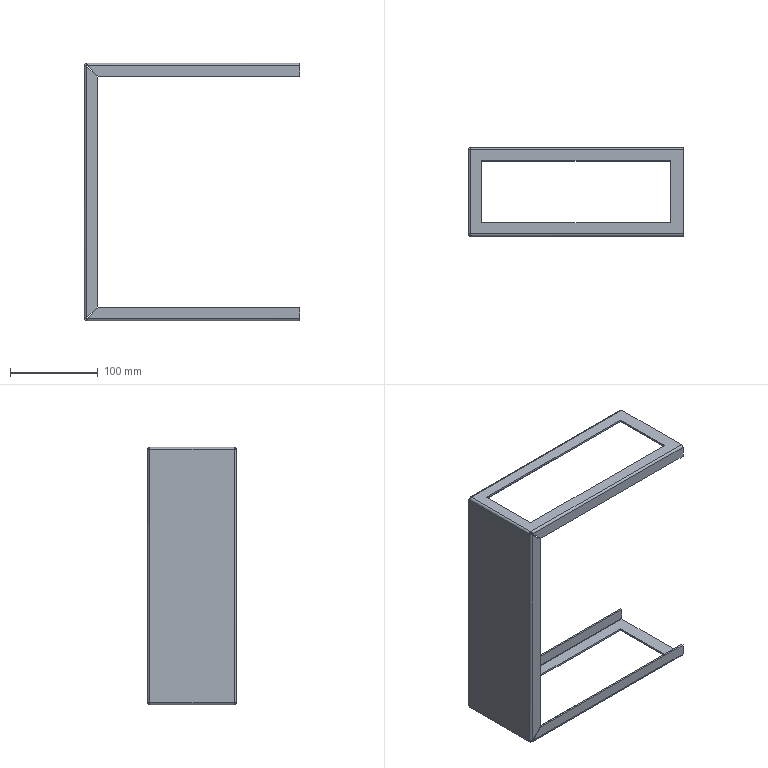Part | SolidWorks | features BaseBody 1 | 1 solid | 78 faces | box 245 x 101 x 293 mm | volume 132791 mm3 | plane 54 | cylinder 16 | spline 8 | commonest cylinder face diameters 1 x8 5 x8